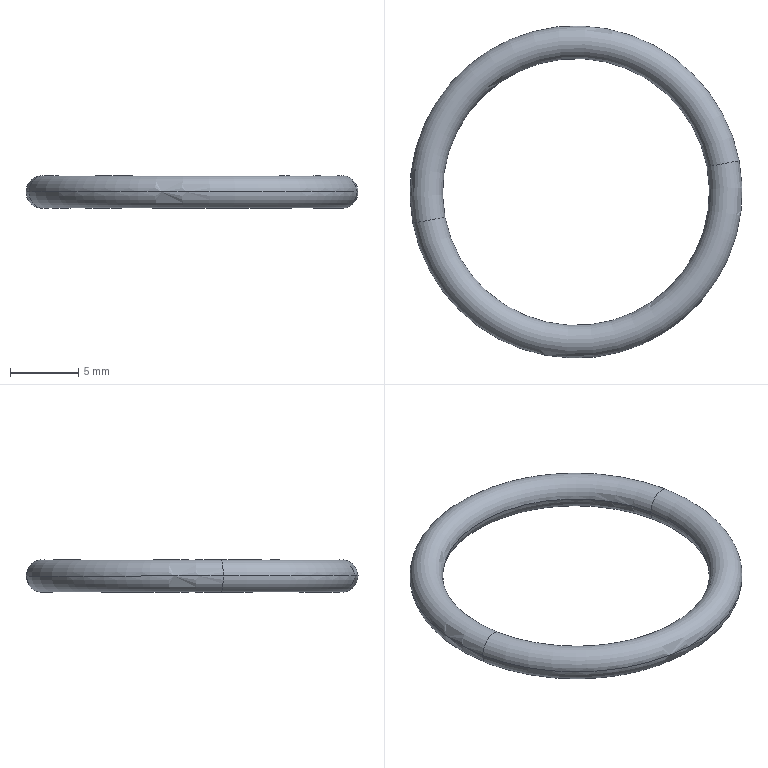Part | SolidWorks | features BaseBody 1 | 1 solid | 4 faces | box 24.4 x 24.4 x 2.4 mm | volume 312.669 mm3 | torus 4
STEP:
#1=CARTESIAN_POINT('',(395.081,104.801,-45.9));
#2=VERTEX_POINT('',#1);
#3=CARTESIAN_POINT('',(392.724,104.349,-45.9));
#4=VERTEX_POINT('',#3);
#5=CARTESIAN_POINT('',(393.903,104.575,-45.9));
#6=DIRECTION('',(0.1886,-0.982,0.));
#7=DIRECTION('',(0.982,0.1886,0.));
#8=AXIS2_PLACEMENT_3D('',#5,#6,#7);
#9=CIRCLE('',#8,1.2);
#10=EDGE_CURVE('',#2,#4,#9,.T.);
#11=ORIENTED_EDGE('',*,*,#10,.F.);
#12=CARTESIAN_POINT('',(371.119,100.199,-45.9));
#13=VERTEX_POINT('',#12);
#14=CARTESIAN_POINT('',(383.1,102.5,-45.9));
#15=DIRECTION('',(0.,0.,1.));
#16=DIRECTION('',(0.,-1.,0.));
#17=AXIS2_PLACEMENT_3D('',#14,#15,#16);
#18=CIRCLE('',#17,12.2);
#19=EDGE_CURVE('',#2,#13,#18,.T.);
#20=ORIENTED_EDGE('',*,*,#19,.T.);
#21=CARTESIAN_POINT('',(373.476,100.651,-45.9));
#22=VERTEX_POINT('',#21);
#23=CARTESIAN_POINT('',(372.297,100.425,-45.9));
#24=DIRECTION('',(-0.1886,0.982,0.));
#25=DIRECTION('',(-0.982,-0.1886,0.));
#26=AXIS2_PLACEMENT_3D('',#23,#24,#25);
#27=CIRCLE('',#26,1.2);
#28=EDGE_CURVE('',#13,#22,#27,.T.);
#29=ORIENTED_EDGE('',*,*,#28,.T.);
#30=CARTESIAN_POINT('',(383.1,102.5,-45.9));
#31=DIRECTION('',(0.,0.,1.));
#32=DIRECTION('',(0.,-1.,0.));
#33=AXIS2_PLACEMENT_3D('',#30,#31,#32);
#34=CIRCLE('',#33,9.8);
#35=EDGE_CURVE('',#4,#22,#34,.T.);
#36=ORIENTED_EDGE('',*,*,#35,.F.);
#37=EDGE_LOOP('',(#11,#20,#29,#36));
#38=FACE_OUTER_BOUND('',#37,.T.);
#39=CARTESIAN_POINT('',(383.1,102.5,-45.9));
#40=DIRECTION('',(0.,0.,1.));
#41=DIRECTION('',(-0.982,-0.1886,0.));
#42=AXIS2_PLACEMENT_3D('',#39,#40,#41);
#43=TOROIDAL_SURFACE('',#42,11.,1.2);
#44=ADVANCED_FACE('',(#38),#43,.T.);
#45=ORIENTED_EDGE('',*,*,#28,.F.);
#46=CARTESIAN_POINT('',(383.1,102.5,-45.9));
#47=DIRECTION('',(0.,0.,1.));
#48=DIRECTION('',(0.,-1.,0.));
#49=AXIS2_PLACEMENT_3D('',#46,#47,#48);
#50=CIRCLE('',#49,12.2);
#51=EDGE_CURVE('',#13,#2,#50,.T.);
#52=ORIENTED_EDGE('',*,*,#51,.T.);
#53=ORIENTED_EDGE('',*,*,#10,.T.);
#54=CARTESIAN_POINT('',(383.1,102.5,-45.9));
#55=DIRECTION('',(0.,0.,1.));
#56=DIRECTION('',(0.,-1.,0.));
#57=AXIS2_PLACEMENT_3D('',#54,#55,#56);
#58=CIRCLE('',#57,9.8);
#59=EDGE_CURVE('',#22,#4,#58,.T.);
#60=ORIENTED_EDGE('',*,*,#59,.F.);
#61=EDGE_LOOP('',(#45,#52,#53,#60));
#62=FACE_OUTER_BOUND('',#61,.T.);
#63=CARTESIAN_POINT('',(383.1,102.5,-45.9));
#64=DIRECTION('',(0.,0.,1.));
#65=DIRECTION('',(-0.982,-0.1886,0.));
#66=AXIS2_PLACEMENT_3D('',#63,#64,#65);
#67=TOROIDAL_SURFACE('',#66,11.,1.2);
#68=ADVANCED_FACE('',(#62),#67,.T.);
#69=ORIENTED_EDGE('',*,*,#51,.F.);
#70=CARTESIAN_POINT('',(372.297,100.425,-45.9));
#71=DIRECTION('',(-0.1886,0.982,0.));
#72=DIRECTION('',(-0.982,-0.1886,0.));
#73=AXIS2_PLACEMENT_3D('',#70,#71,#72);
#74=CIRCLE('',#73,1.2);
#75=EDGE_CURVE('',#22,#13,#74,.T.);
#76=ORIENTED_EDGE('',*,*,#75,.F.);
#77=ORIENTED_EDGE('',*,*,#59,.T.);
#78=CARTESIAN_POINT('',(393.903,104.575,-45.9));
#79=DIRECTION('',(0.1886,-0.982,0.));
#80=DIRECTION('',(0.982,0.1886,0.));
#81=AXIS2_PLACEMENT_3D('',#78,#79,#80);
#82=CIRCLE('',#81,1.2);
#83=EDGE_CURVE('',#4,#2,#82,.T.);
#84=ORIENTED_EDGE('',*,*,#83,.T.);
#85=EDGE_LOOP('',(#69,#76,#77,#84));
#86=FACE_OUTER_BOUND('',#85,.T.);
#87=CARTESIAN_POINT('',(383.1,102.5,-45.9));
#88=DIRECTION('',(0.,0.,1.));
#89=DIRECTION('',(-0.982,-0.1886,0.));
#90=AXIS2_PLACEMENT_3D('',#87,#88,#89);
#91=TOROIDAL_SURFACE('',#90,11.,1.2);
#92=ADVANCED_FACE('',(#86),#91,.T.);
#93=ORIENTED_EDGE('',*,*,#19,.F.);
#94=ORIENTED_EDGE('',*,*,#83,.F.);
#95=ORIENTED_EDGE('',*,*,#35,.T.);
#96=ORIENTED_EDGE('',*,*,#75,.T.);
#97=EDGE_LOOP('',(#93,#94,#95,#96));
#98=FACE_OUTER_BOUND('',#97,.T.);
#99=CARTESIAN_POINT('',(383.1,102.5,-45.9));
#100=DIRECTION('',(0.,0.,1.));
#101=DIRECTION('',(-0.982,-0.1886,0.));
#102=AXIS2_PLACEMENT_3D('',#99,#100,#101);
#103=TOROIDAL_SURFACE('',#102,11.,1.2);
#104=ADVANCED_FACE('',(#98),#103,.T.);
#105=CLOSED_SHELL('',(#44,#68,#92,#104));
#106=MANIFOLD_SOLID_BREP('',#105);
#107=CARTESIAN_POINT('',(0.,0.,0.));
#108=DIRECTION('',(0.,0.,1.));
#109=DIRECTION('',(1.,0.,0.));
#110=AXIS2_PLACEMENT_3D('',#107,#108,#109);
#111=(LENGTH_UNIT()NAMED_UNIT(*)SI_UNIT(.MILLI.,.METRE.));
#112=UNCERTAINTY_MEASURE_WITH_UNIT(LENGTH_MEASURE(0.00001),#111,'','');
#113=(NAMED_UNIT(*)PLANE_ANGLE_UNIT()SI_UNIT($,.RADIAN.));
#114=(NAMED_UNIT(*)SI_UNIT($,.STERADIAN.)SOLID_ANGLE_UNIT());
#115=(GEOMETRIC_REPRESENTATION_CONTEXT(3)GLOBAL_UNCERTAINTY_ASSIGNED_CONTEXT((#112))GLOBAL_UNIT_ASSIGNED_CONTEXT((#111,#113,#114))REPRESENTATION_CONTEXT('',''));
#116=ADVANCED_BREP_SHAPE_REPRESENTATION('',(#106,#110),#115);